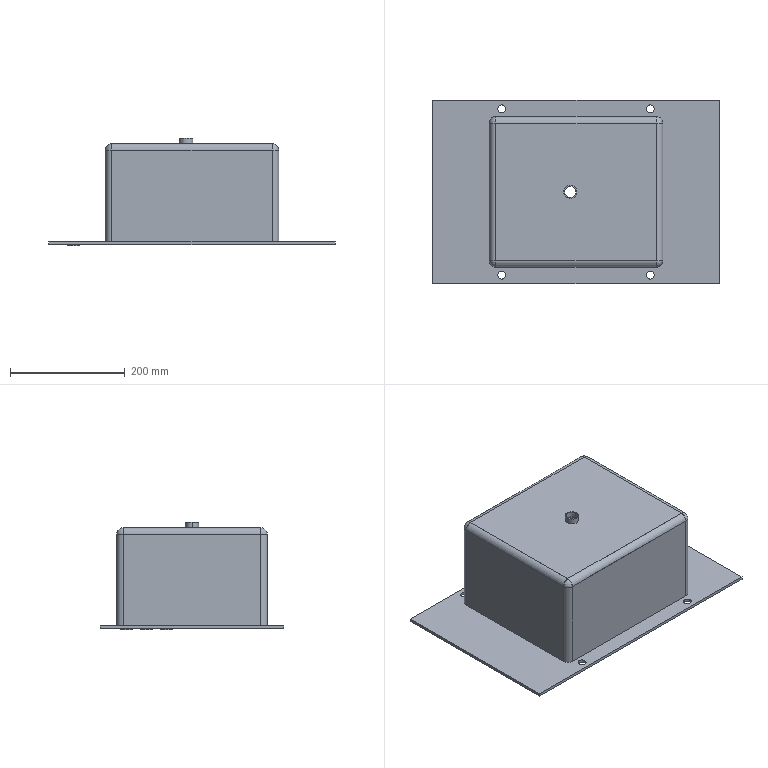Part | SolidWorks | features ICE 5, Fillet 2, Extrusion 1 | 1 solid | 65 faces | box 500 x 320 x 188.5 mm | volume 804078 mm3 | cylinder 36 | plane 21 | sphere 8 | commonest cylinder face diameters 20 x10 14 x8 23 x8 21.332 x6 19.935 x2 22.935 x2